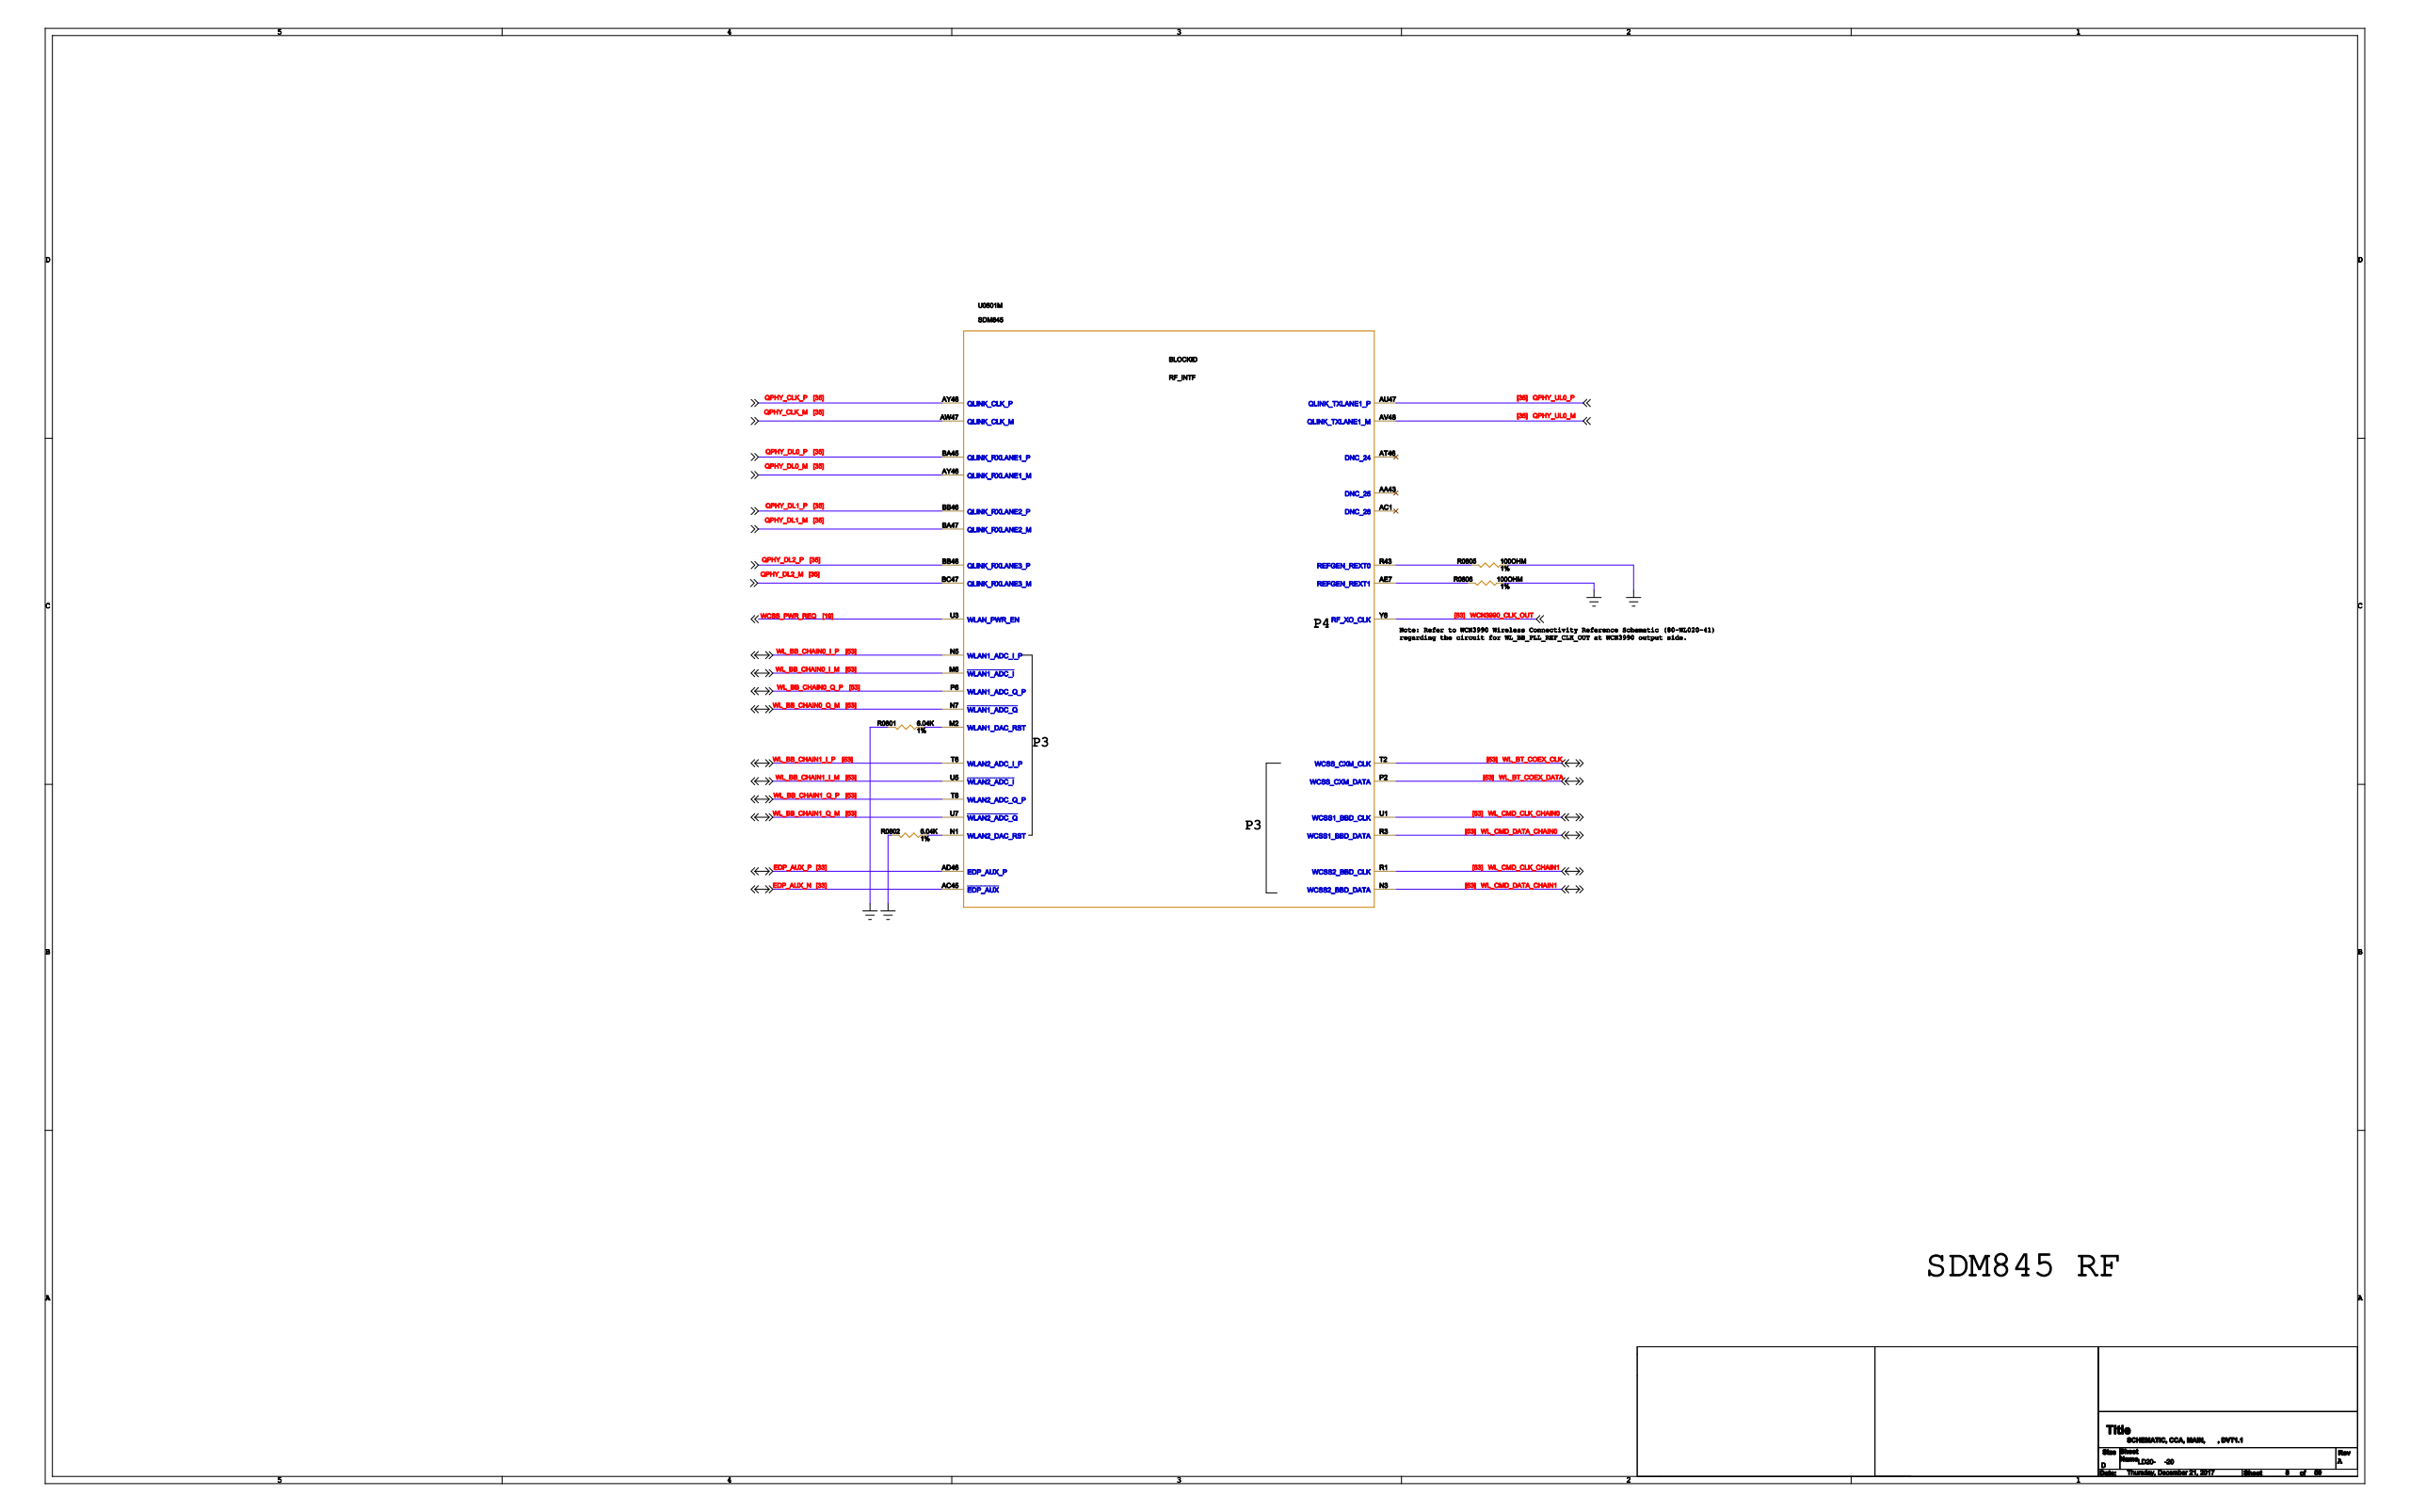Circuit board | Cadence Allegro | 1520 parts | 1149 nets | one sheet of the schematic
Parts on this sheet (reference | value | footprint):
R0801 | 6.04K | 2P0201R
R0802 | 6.04K | 2P0201R
R0805 | 100OHM | 2P0201R
R0806 | 100OHM | 2P0201R
U0501 | SDM845 | 914PGA490X490B138D45
Nets of these parts (net: part-pin ...):
GND: R0801-1 R0802-1 R0805-2 R0806-2 U0501-P4
QPHY_CLK_M: U0501-AW47
QPHY_CLK_P: U0501-AY48
QPHY_DL0_M: U0501-AY46
QPHY_DL0_P: U0501-BA45
QPHY_DL1_M: U0501-BA47
QPHY_DL1_P: U0501-BB46
QPHY_DL2_M: U0501-BC47
QPHY_DL2_P: U0501-BB48
QPHY_UL0_M: U0501-AV48
QPHY_UL0_P: U0501-AU47
EDP_AUX_P: U0501-AD46
EDP_AUX_N: U0501-AC45
WL_CMD_DATA_CHAIN0: U0501-R3
WL_CMD_DATA_CHAIN1: U0501-N3
WL_CMD_CLK_CHAIN0: U0501-U1
WL_CMD_CLK_CHAIN1: U0501-R1
WCN3990_CLK_OUT: U0501-Y6
N34635013: R0801-2 U0501-M2
N34635011: R0802-2 U0501-N1
N34635131: R0805-1 U0501-R43
N34635133: R0806-1 U0501-AE7
WL_BT_COEX_CLK: U0501-T2
WL_BT_COEX_DATA: U0501-P2
WL_BB_CHAIN0_I_P: U0501-N5
WL_BB_CHAIN0_Q_P: U0501-P6
WL_BB_CHAIN1_I_P: U0501-T6
WL_BB_CHAIN1_Q_P: U0501-T8
WCSS_PWR_REQ: U0501-U3
WL_BB_CHAIN0_I_M: U0501-M6
WL_BB_CHAIN0_Q_M: U0501-N7
WL_BB_CHAIN1_I_M: U0501-U5
WL_BB_CHAIN1_Q_M: U0501-U7